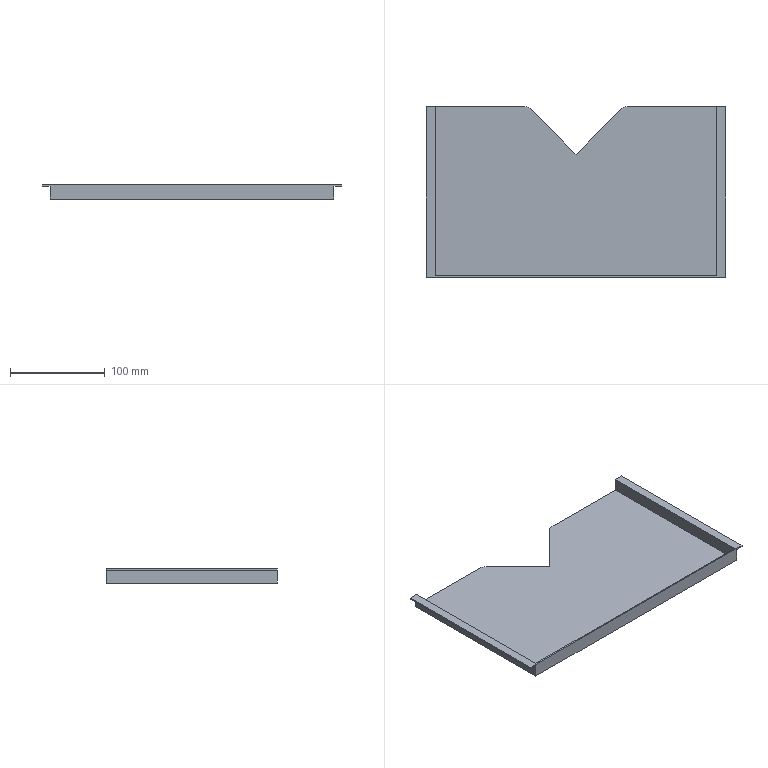Part | STEP file | 1 solid | 19 faces | box 316 x 180 x 15 mm | volume 94868 mm3 | plane 17 | cylinder 2 | commonest cylinder face diameters 20 x2
STEP:
#1=CARTESIAN_POINT('',(0.,0.,0.));
#2=DIRECTION('',(0.,0.,1.));
#3=DIRECTION('',(1.,0.,0.));
#4=AXIS2_PLACEMENT_3D('',#1,#2,#3);
#5=CARTESIAN_POINT('',(150.,90.,-15.));
#6=VERTEX_POINT('',#5);
#7=CARTESIAN_POINT('',(54.142,90.,-15.));
#8=VERTEX_POINT('',#7);
#9=CARTESIAN_POINT('',(158.,90.,-15.));
#10=DIRECTION('',(-1.,0.,0.));
#11=VECTOR('',#10,1.);
#12=LINE('',#9,#11);
#13=CARTESIAN_POINT('',(158.,-90.,-15.));
#14=DIRECTION('',(0.,0.,1.));
#15=DIRECTION('',(1.,0.,0.));
#16=AXIS2_PLACEMENT_3D('',#13,#14,#15);
#17=PLANE('',#16);
#18=CARTESIAN_POINT('',(0.,180.));
#19=DIRECTION('',(-1.,0.));
#20=VECTOR('',#19,1.);
#21=LINE('',#18,#20);
#22=(GEOMETRIC_REPRESENTATION_CONTEXT(2)PARAMETRIC_REPRESENTATION_CONTEXT()REPRESENTATION_CONTEXT('',''));
#23=DEFINITIONAL_REPRESENTATION('',(#21),#22);
#24=PCURVE('',#17,#23);
#25=CARTESIAN_POINT('',(-158.,90.,-15.));
#26=DIRECTION('',(0.,1.,0.));
#27=DIRECTION('',(0.,0.,1.));
#28=AXIS2_PLACEMENT_3D('',#25,#26,#27);
#29=PLANE('',#28);
#30=CARTESIAN_POINT('',(0.,316.));
#31=DIRECTION('',(0.,-1.));
#32=VECTOR('',#31,1.);
#33=LINE('',#30,#32);
#34=(GEOMETRIC_REPRESENTATION_CONTEXT(2)PARAMETRIC_REPRESENTATION_CONTEXT()REPRESENTATION_CONTEXT('',''));
#35=DEFINITIONAL_REPRESENTATION('',(#33),#34);
#36=PCURVE('',#29,#35);
#37=SURFACE_CURVE('',#12,(#24,#36),.PCURVE_S1.);
#38=EDGE_CURVE('',#6,#8,#37,.T.);
#39=ORIENTED_EDGE('',*,*,#38,.F.);
#40=CARTESIAN_POINT('',(150.,-90.,-15.));
#41=VERTEX_POINT('',#40);
#42=CARTESIAN_POINT('',(150.,-90.,-15.));
#43=DIRECTION('',(0.,1.,0.));
#44=VECTOR('',#43,1.);
#45=LINE('',#42,#44);
#46=CARTESIAN_POINT('',(-8.,0.));
#47=DIRECTION('',(0.,1.));
#48=VECTOR('',#47,1.);
#49=LINE('',#46,#48);
#50=(GEOMETRIC_REPRESENTATION_CONTEXT(2)PARAMETRIC_REPRESENTATION_CONTEXT()REPRESENTATION_CONTEXT('',''));
#51=DEFINITIONAL_REPRESENTATION('',(#49),#50);
#52=PCURVE('',#17,#51);
#53=CARTESIAN_POINT('',(150.,109.,-15.));
#54=DIRECTION('',(-1.,0.,0.));
#55=DIRECTION('',(0.,0.,1.));
#56=AXIS2_PLACEMENT_3D('',#53,#54,#55);
#57=PLANE('',#56);
#58=CARTESIAN_POINT('',(0.,-199.));
#59=DIRECTION('',(0.,1.));
#60=VECTOR('',#59,1.);
#61=LINE('',#58,#60);
#62=(GEOMETRIC_REPRESENTATION_CONTEXT(2)PARAMETRIC_REPRESENTATION_CONTEXT()REPRESENTATION_CONTEXT('',''));
#63=DEFINITIONAL_REPRESENTATION('',(#61),#62);
#64=PCURVE('',#57,#63);
#65=SURFACE_CURVE('',#45,(#52,#64),.PCURVE_S1.);
#66=EDGE_CURVE('',#41,#6,#65,.T.);
#67=ORIENTED_EDGE('',*,*,#66,.F.);
#68=CARTESIAN_POINT('',(-150.,-90.,-15.));
#69=VERTEX_POINT('',#68);
#70=CARTESIAN_POINT('',(158.,-90.,-15.));
#71=DIRECTION('',(1.,0.,0.));
#72=VECTOR('',#71,1.);
#73=LINE('',#70,#72);
#74=CARTESIAN_POINT('',(0.,0.));
#75=DIRECTION('',(1.,0.));
#76=VECTOR('',#75,1.);
#77=LINE('',#74,#76);
#78=(GEOMETRIC_REPRESENTATION_CONTEXT(2)PARAMETRIC_REPRESENTATION_CONTEXT()REPRESENTATION_CONTEXT('',''));
#79=DEFINITIONAL_REPRESENTATION('',(#77),#78);
#80=PCURVE('',#17,#79);
#81=CARTESIAN_POINT('',(-158.,-90.,-15.));
#82=DIRECTION('',(0.,-1.,0.));
#83=DIRECTION('',(0.,0.,-1.));
#84=AXIS2_PLACEMENT_3D('',#81,#82,#83);
#85=PLANE('',#84);
#86=CARTESIAN_POINT('',(0.,316.));
#87=DIRECTION('',(0.,1.));
#88=VECTOR('',#87,1.);
#89=LINE('',#86,#88);
#90=(GEOMETRIC_REPRESENTATION_CONTEXT(2)PARAMETRIC_REPRESENTATION_CONTEXT()REPRESENTATION_CONTEXT('',''));
#91=DEFINITIONAL_REPRESENTATION('',(#89),#90);
#92=PCURVE('',#85,#91);
#93=SURFACE_CURVE('',#73,(#80,#92),.PCURVE_S1.);
#94=EDGE_CURVE('',#69,#41,#93,.T.);
#95=ORIENTED_EDGE('',*,*,#94,.F.);
#96=CARTESIAN_POINT('',(-150.,90.,-15.));
#97=VERTEX_POINT('',#96);
#98=CARTESIAN_POINT('',(-150.,-90.,-15.));
#99=DIRECTION('',(0.,-1.,0.));
#100=VECTOR('',#99,1.);
#101=LINE('',#98,#100);
#102=CARTESIAN_POINT('',(-308.,0.));
#103=DIRECTION('',(0.,-1.));
#104=VECTOR('',#103,1.);
#105=LINE('',#102,#104);
#106=(GEOMETRIC_REPRESENTATION_CONTEXT(2)PARAMETRIC_REPRESENTATION_CONTEXT()REPRESENTATION_CONTEXT('',''));
#107=DEFINITIONAL_REPRESENTATION('',(#105),#106);
#108=PCURVE('',#17,#107);
#109=CARTESIAN_POINT('',(-150.,109.,-15.));
#110=DIRECTION('',(-1.,0.,0.));
#111=DIRECTION('',(0.,0.,1.));
#112=AXIS2_PLACEMENT_3D('',#109,#110,#111);
#113=PLANE('',#112);
#114=CARTESIAN_POINT('',(0.,-199.));
#115=DIRECTION('',(0.,-1.));
#116=VECTOR('',#115,1.);
#117=LINE('',#114,#116);
#118=(GEOMETRIC_REPRESENTATION_CONTEXT(2)PARAMETRIC_REPRESENTATION_CONTEXT()REPRESENTATION_CONTEXT('',''));
#119=DEFINITIONAL_REPRESENTATION('',(#117),#118);
#120=PCURVE('',#113,#119);
#121=SURFACE_CURVE('',#101,(#108,#120),.PCURVE_S1.);
#122=EDGE_CURVE('',#97,#69,#121,.T.);
#123=ORIENTED_EDGE('',*,*,#122,.F.);
#124=CARTESIAN_POINT('',(-54.142,90.,-15.));
#125=VERTEX_POINT('',#124);
#126=CARTESIAN_POINT('',(158.,90.,-15.));
#127=DIRECTION('',(-1.,0.,0.));
#128=VECTOR('',#127,1.);
#129=LINE('',#126,#128);
#130=CARTESIAN_POINT('',(0.,180.));
#131=DIRECTION('',(-1.,0.));
#132=VECTOR('',#131,1.);
#133=LINE('',#130,#132);
#134=(GEOMETRIC_REPRESENTATION_CONTEXT(2)PARAMETRIC_REPRESENTATION_CONTEXT()REPRESENTATION_CONTEXT('',''));
#135=DEFINITIONAL_REPRESENTATION('',(#133),#134);
#136=PCURVE('',#17,#135);
#137=CARTESIAN_POINT('',(-158.,90.,-15.));
#138=DIRECTION('',(0.,1.,0.));
#139=DIRECTION('',(0.,0.,1.));
#140=AXIS2_PLACEMENT_3D('',#137,#138,#139);
#141=PLANE('',#140);
#142=CARTESIAN_POINT('',(0.,316.));
#143=DIRECTION('',(0.,-1.));
#144=VECTOR('',#143,1.);
#145=LINE('',#142,#144);
#146=(GEOMETRIC_REPRESENTATION_CONTEXT(2)PARAMETRIC_REPRESENTATION_CONTEXT()REPRESENTATION_CONTEXT('',''));
#147=DEFINITIONAL_REPRESENTATION('',(#145),#146);
#148=PCURVE('',#141,#147);
#149=SURFACE_CURVE('',#129,(#136,#148),.PCURVE_S1.);
#150=EDGE_CURVE('',#125,#97,#149,.T.);
#151=ORIENTED_EDGE('',*,*,#150,.F.);
#152=CARTESIAN_POINT('',(-47.071,87.071,-15.));
#153=VERTEX_POINT('',#152);
#154=CARTESIAN_POINT('',(-54.142,80.,-15.));
#155=DIRECTION('',(0.,0.,1.));
#156=DIRECTION('',(1.,0.,0.));
#157=AXIS2_PLACEMENT_3D('',#154,#155,#156);
#158=CIRCLE('',#157,10.);
#159=CARTESIAN_POINT('',(-212.142,170.));
#160=DIRECTION('',(1.,0.));
#161=AXIS2_PLACEMENT_2D('',#159,#160);
#162=CIRCLE('',#161,10.);
#163=(GEOMETRIC_REPRESENTATION_CONTEXT(2)PARAMETRIC_REPRESENTATION_CONTEXT()REPRESENTATION_CONTEXT('',''));
#164=DEFINITIONAL_REPRESENTATION('',(#162),#163);
#165=PCURVE('',#17,#164);
#166=CARTESIAN_POINT('',(-54.142,80.,-488.724));
#167=DIRECTION('',(0.,0.,1.));
#168=DIRECTION('',(1.,0.,0.));
#169=AXIS2_PLACEMENT_3D('',#166,#167,#168);
#170=CYLINDRICAL_SURFACE('',#169,10.);
#171=CARTESIAN_POINT('',(0.,473.724));
#172=DIRECTION('',(1.,0.));
#173=VECTOR('',#172,1.);
#174=LINE('',#171,#173);
#175=(GEOMETRIC_REPRESENTATION_CONTEXT(2)PARAMETRIC_REPRESENTATION_CONTEXT()REPRESENTATION_CONTEXT('',''));
#176=DEFINITIONAL_REPRESENTATION('',(#174),#175);
#177=PCURVE('',#170,#176);
#178=SURFACE_CURVE('',#158,(#165,#177),.PCURVE_S1.);
#179=EDGE_CURVE('',#153,#125,#178,.T.);
#180=ORIENTED_EDGE('',*,*,#179,.F.);
#181=CARTESIAN_POINT('',(0.,40.,-15.));
#182=VERTEX_POINT('',#181);
#183=CARTESIAN_POINT('',(0.,40.,-15.));
#184=DIRECTION('',(-0.7071,0.7071,0.));
#185=VECTOR('',#184,1.);
#186=LINE('',#183,#185);
#187=CARTESIAN_POINT('',(-158.,130.));
#188=DIRECTION('',(-0.7071,0.7071));
#189=VECTOR('',#188,1.);
#190=LINE('',#187,#189);
#191=(GEOMETRIC_REPRESENTATION_CONTEXT(2)PARAMETRIC_REPRESENTATION_CONTEXT()REPRESENTATION_CONTEXT('',''));
#192=DEFINITIONAL_REPRESENTATION('',(#190),#191);
#193=PCURVE('',#17,#192);
#194=CARTESIAN_POINT('',(0.,40.,-488.724));
#195=DIRECTION('',(-0.7071,-0.7071,0.));
#196=DIRECTION('',(0.7071,-0.7071,0.));
#197=AXIS2_PLACEMENT_3D('',#194,#195,#196);
#198=PLANE('',#197);
#199=CARTESIAN_POINT('',(0.,473.724));
#200=DIRECTION('',(-1.,0.));
#201=VECTOR('',#200,1.);
#202=LINE('',#199,#201);
#203=(GEOMETRIC_REPRESENTATION_CONTEXT(2)PARAMETRIC_REPRESENTATION_CONTEXT()REPRESENTATION_CONTEXT('',''));
#204=DEFINITIONAL_REPRESENTATION('',(#202),#203);
#205=PCURVE('',#198,#204);
#206=SURFACE_CURVE('',#186,(#193,#205),.PCURVE_S1.);
#207=EDGE_CURVE('',#182,#153,#206,.T.);
#208=ORIENTED_EDGE('',*,*,#207,.F.);
#209=CARTESIAN_POINT('',(47.071,87.071,-15.));
#210=VERTEX_POINT('',#209);
#211=CARTESIAN_POINT('',(47.071,87.071,-15.));
#212=DIRECTION('',(-0.7071,-0.7071,0.));
#213=VECTOR('',#212,1.);
#214=LINE('',#211,#213);
#215=CARTESIAN_POINT('',(-110.929,177.071));
#216=DIRECTION('',(-0.7071,-0.7071));
#217=VECTOR('',#216,1.);
#218=LINE('',#215,#217);
#219=(GEOMETRIC_REPRESENTATION_CONTEXT(2)PARAMETRIC_REPRESENTATION_CONTEXT()REPRESENTATION_CONTEXT('',''));
#220=DEFINITIONAL_REPRESENTATION('',(#218),#219);
#221=PCURVE('',#17,#220);
#222=CARTESIAN_POINT('',(0.,40.,-488.724));
#223=DIRECTION('',(0.7071,-0.7071,0.));
#224=DIRECTION('',(0.7071,0.7071,0.));
#225=AXIS2_PLACEMENT_3D('',#222,#223,#224);
#226=PLANE('',#225);
#227=CARTESIAN_POINT('',(66.569,473.724));
#228=DIRECTION('',(-1.,0.));
#229=VECTOR('',#228,1.);
#230=LINE('',#227,#229);
#231=(GEOMETRIC_REPRESENTATION_CONTEXT(2)PARAMETRIC_REPRESENTATION_CONTEXT()REPRESENTATION_CONTEXT('',''));
#232=DEFINITIONAL_REPRESENTATION('',(#230),#231);
#233=PCURVE('',#226,#232);
#234=SURFACE_CURVE('',#214,(#221,#233),.PCURVE_S1.);
#235=EDGE_CURVE('',#210,#182,#234,.T.);
#236=ORIENTED_EDGE('',*,*,#235,.F.);
#237=CARTESIAN_POINT('',(54.142,80.,-15.));
#238=DIRECTION('',(0.,0.,1.));
#239=DIRECTION('',(1.,0.,0.));
#240=AXIS2_PLACEMENT_3D('',#237,#238,#239);
#241=CIRCLE('',#240,10.);
#242=CARTESIAN_POINT('',(-103.858,170.));
#243=DIRECTION('',(1.,0.));
#244=AXIS2_PLACEMENT_2D('',#242,#243);
#245=CIRCLE('',#244,10.);
#246=(GEOMETRIC_REPRESENTATION_CONTEXT(2)PARAMETRIC_REPRESENTATION_CONTEXT()REPRESENTATION_CONTEXT('',''));
#247=DEFINITIONAL_REPRESENTATION('',(#245),#246);
#248=PCURVE('',#17,#247);
#249=CARTESIAN_POINT('',(54.142,80.,-15.));
#250=DIRECTION('',(0.,0.,1.));
#251=DIRECTION('',(1.,0.,0.));
#252=AXIS2_PLACEMENT_3D('',#249,#250,#251);
#253=CYLINDRICAL_SURFACE('',#252,10.);
#254=CARTESIAN_POINT('',(0.,0.));
#255=DIRECTION('',(1.,0.));
#256=VECTOR('',#255,1.);
#257=LINE('',#254,#256);
#258=(GEOMETRIC_REPRESENTATION_CONTEXT(2)PARAMETRIC_REPRESENTATION_CONTEXT()REPRESENTATION_CONTEXT('',''));
#259=DEFINITIONAL_REPRESENTATION('',(#257),#258);
#260=PCURVE('',#253,#259);
#261=SURFACE_CURVE('',#241,(#248,#260),.PCURVE_S1.);
#262=EDGE_CURVE('',#8,#210,#261,.T.);
#263=ORIENTED_EDGE('',*,*,#262,.F.);
#264=EDGE_LOOP('',(#39,#67,#95,#123,#151,#180,#208,#236,#263));
#265=FACE_BOUND('',#264,.T.);
#266=ADVANCED_FACE('',(#265),#17,.F.);
#267=ORIENTED_EDGE('',*,*,#262,.T.);
#268=CARTESIAN_POINT('',(47.071,87.071,-13.5));
#269=VERTEX_POINT('',#268);
#270=CARTESIAN_POINT('',(47.071,87.071,-15.));
#271=DIRECTION('',(0.,0.,1.));
#272=VECTOR('',#271,1.);
#273=LINE('',#270,#272);
#274=CARTESIAN_POINT('',(2.356,0.));
#275=DIRECTION('',(0.,1.));
#276=VECTOR('',#275,1.);
#277=LINE('',#274,#276);
#278=(GEOMETRIC_REPRESENTATION_CONTEXT(2)PARAMETRIC_REPRESENTATION_CONTEXT()REPRESENTATION_CONTEXT('',''));
#279=DEFINITIONAL_REPRESENTATION('',(#277),#278);
#280=PCURVE('',#253,#279);
#281=CARTESIAN_POINT('',(66.569,473.724));
#282=DIRECTION('',(0.,1.));
#283=VECTOR('',#282,1.);
#284=LINE('',#281,#283);
#285=(GEOMETRIC_REPRESENTATION_CONTEXT(2)PARAMETRIC_REPRESENTATION_CONTEXT()REPRESENTATION_CONTEXT('',''));
#286=DEFINITIONAL_REPRESENTATION('',(#284),#285);
#287=PCURVE('',#226,#286);
#288=SURFACE_CURVE('',#273,(#280,#287),.PCURVE_S1.);
#289=EDGE_CURVE('',#210,#269,#288,.T.);
#290=ORIENTED_EDGE('',*,*,#289,.T.);
#291=CARTESIAN_POINT('',(54.142,90.,-13.5));
#292=VERTEX_POINT('',#291);
#293=CARTESIAN_POINT('',(54.142,80.,-13.5));
#294=DIRECTION('',(0.,0.,-1.));
#295=DIRECTION('',(1.,0.,0.));
#296=AXIS2_PLACEMENT_3D('',#293,#294,#295);
#297=CIRCLE('',#296,10.);
#298=CARTESIAN_POINT('',(6.283,1.5));
#299=DIRECTION('',(-1.,0.));
#300=VECTOR('',#299,1.);
#301=LINE('',#298,#300);
#302=(GEOMETRIC_REPRESENTATION_CONTEXT(2)PARAMETRIC_REPRESENTATION_CONTEXT()REPRESENTATION_CONTEXT('',''));
#303=DEFINITIONAL_REPRESENTATION('',(#301),#302);
#304=PCURVE('',#253,#303);
#305=CARTESIAN_POINT('',(158.,-90.,-13.5));
#306=DIRECTION('',(0.,0.,1.));
#307=DIRECTION('',(1.,0.,0.));
#308=AXIS2_PLACEMENT_3D('',#305,#306,#307);
#309=PLANE('',#308);
#310=CARTESIAN_POINT('',(-93.858,170.));
#311=CARTESIAN_POINT('',(-93.858,152.679));
#312=CARTESIAN_POINT('',(-108.858,161.34));
#313=CARTESIAN_POINT('',(-123.858,170.));
#314=CARTESIAN_POINT('',(-108.858,178.66));
#315=CARTESIAN_POINT('',(-93.858,187.321));
#316=CARTESIAN_POINT('',(-93.858,170.));
#317=(BOUNDED_CURVE()B_SPLINE_CURVE(2,(#310,#311,#312,#313,#314,#315,#316),.UNSPECIFIED.,.T.,.F.)B_SPLINE_CURVE_WITH_KNOTS((1,2,2,2,2,1),(-2.094,0.,2.094,4.189,6.283,8.378),.UNSPECIFIED.)CURVE()GEOMETRIC_REPRESENTATION_ITEM()RATIONAL_B_SPLINE_CURVE((1.,0.5,1.,0.5,1.,0.5,1.))REPRESENTATION_ITEM(''));
#318=(GEOMETRIC_REPRESENTATION_CONTEXT(2)PARAMETRIC_REPRESENTATION_CONTEXT()REPRESENTATION_CONTEXT('',''));
#319=DEFINITIONAL_REPRESENTATION('',(#317),#318);
#320=PCURVE('',#309,#319);
#321=SURFACE_CURVE('',#297,(#304,#320),.PCURVE_S1.);
#322=EDGE_CURVE('',#269,#292,#321,.T.);
#323=ORIENTED_EDGE('',*,*,#322,.T.);
#324=CARTESIAN_POINT('',(54.142,90.,-15.));
#325=DIRECTION('',(0.,0.,-1.));
#326=VECTOR('',#325,1.);
#327=LINE('',#324,#326);
#328=CARTESIAN_POINT('',(1.571,0.));
#329=DIRECTION('',(0.,-1.));
#330=VECTOR('',#329,1.);
#331=LINE('',#328,#330);
#332=(GEOMETRIC_REPRESENTATION_CONTEXT(2)PARAMETRIC_REPRESENTATION_CONTEXT()REPRESENTATION_CONTEXT('',''));
#333=DEFINITIONAL_REPRESENTATION('',(#331),#332);
#334=PCURVE('',#253,#333);
#335=CARTESIAN_POINT('',(0.,212.142));
#336=DIRECTION('',(-1.,0.));
#337=VECTOR('',#336,1.);
#338=LINE('',#335,#337);
#339=(GEOMETRIC_REPRESENTATION_CONTEXT(2)PARAMETRIC_REPRESENTATION_CONTEXT()REPRESENTATION_CONTEXT('',''));
#340=DEFINITIONAL_REPRESENTATION('',(#338),#339);
#341=PCURVE('',#29,#340);
#342=SURFACE_CURVE('',#327,(#334,#341),.PCURVE_S1.);
#343=EDGE_CURVE('',#292,#8,#342,.T.);
#344=ORIENTED_EDGE('',*,*,#343,.T.);
#345=EDGE_LOOP('',(#267,#290,#323,#344));
#346=FACE_BOUND('',#345,.T.);
#347=ADVANCED_FACE('',(#346),#253,.T.);
#348=CARTESIAN_POINT('',(148.5,90.,0.));
#349=VERTEX_POINT('',#348);
#350=CARTESIAN_POINT('',(158.,90.,0.));
#351=VERTEX_POINT('',#350);
#352=CARTESIAN_POINT('',(-158.,90.,0.));
#353=DIRECTION('',(1.,0.,0.));
#354=VECTOR('',#353,1.);
#355=LINE('',#352,#354);
#356=CARTESIAN_POINT('',(15.,0.));
#357=DIRECTION('',(0.,1.));
#358=VECTOR('',#357,1.);
#359=LINE('',#356,#358);
#360=(GEOMETRIC_REPRESENTATION_CONTEXT(2)PARAMETRIC_REPRESENTATION_CONTEXT()REPRESENTATION_CONTEXT('',''));
#361=DEFINITIONAL_REPRESENTATION('',(#359),#360);
#362=PCURVE('',#29,#361);
#363=CARTESIAN_POINT('',(158.,-90.,0.));
#364=DIRECTION('',(0.,0.,1.));
#365=DIRECTION('',(1.,0.,0.));
#366=AXIS2_PLACEMENT_3D('',#363,#364,#365);
#367=PLANE('',#366);
#368=CARTESIAN_POINT('',(-316.,180.));
#369=DIRECTION('',(1.,0.));
#370=VECTOR('',#369,1.);
#371=LINE('',#368,#370);
#372=(GEOMETRIC_REPRESENTATION_CONTEXT(2)PARAMETRIC_REPRESENTATION_CONTEXT()REPRESENTATION_CONTEXT('',''));
#373=DEFINITIONAL_REPRESENTATION('',(#371),#372);
#374=PCURVE('',#367,#373);
#375=SURFACE_CURVE('',#355,(#362,#374),.PCURVE_S1.);
#376=EDGE_CURVE('',#349,#351,#375,.T.);
#377=ORIENTED_EDGE('',*,*,#376,.T.);
#378=CARTESIAN_POINT('',(158.,90.,-1.5));
#379=VERTEX_POINT('',#378);
#380=CARTESIAN_POINT('',(158.,90.,-15.));
#381=DIRECTION('',(0.,0.,1.));
#382=VECTOR('',#381,1.);
#383=LINE('',#380,#382);
#384=CARTESIAN_POINT('',(0.,316.));
#385=DIRECTION('',(1.,0.));
#386=VECTOR('',#385,1.);
#387=LINE('',#384,#386);
#388=(GEOMETRIC_REPRESENTATION_CONTEXT(2)PARAMETRIC_REPRESENTATION_CONTEXT()REPRESENTATION_CONTEXT('',''));
#389=DEFINITIONAL_REPRESENTATION('',(#387),#388);
#390=PCURVE('',#29,#389);
#391=CARTESIAN_POINT('',(158.,90.,-15.));
#392=DIRECTION('',(1.,0.,0.));
#393=DIRECTION('',(0.,0.,-1.));
#394=AXIS2_PLACEMENT_3D('',#391,#392,#393);
#395=PLANE('',#394);
#396=CARTESIAN_POINT('',(0.,0.));
#397=DIRECTION('',(-1.,0.));
#398=VECTOR('',#397,1.);
#399=LINE('',#396,#398);
#400=(GEOMETRIC_REPRESENTATION_CONTEXT(2)PARAMETRIC_REPRESENTATION_CONTEXT()REPRESENTATION_CONTEXT('',''));
#401=DEFINITIONAL_REPRESENTATION('',(#399),#400);
#402=PCURVE('',#395,#401);
#403=SURFACE_CURVE('',#383,(#390,#402),.PCURVE_S1.);
#404=EDGE_CURVE('',#379,#351,#403,.T.);
#405=ORIENTED_EDGE('',*,*,#404,.F.);
#406=CARTESIAN_POINT('',(150.,90.,-1.5));
#407=VERTEX_POINT('',#406);
#408=CARTESIAN_POINT('',(-158.,90.,-1.5));
#409=DIRECTION('',(-1.,0.,0.));
#410=VECTOR('',#409,1.);
#411=LINE('',#408,#410);
#412=CARTESIAN_POINT('',(13.5,0.));
#413=DIRECTION('',(0.,-1.));
#414=VECTOR('',#413,1.);
#415=LINE('',#412,#414);
#416=(GEOMETRIC_REPRESENTATION_CONTEXT(2)PARAMETRIC_REPRESENTATION_CONTEXT()REPRESENTATION_CONTEXT('',''));
#417=DEFINITIONAL_REPRESENTATION('',(#415),#416);
#418=PCURVE('',#29,#417);
#419=CARTESIAN_POINT('',(158.,109.,-1.5));
#420=DIRECTION('',(0.,0.,1.));
#421=DIRECTION('',(1.,0.,0.));
#422=AXIS2_PLACEMENT_3D('',#419,#420,#421);
#423=PLANE('',#422);
#424=CARTESIAN_POINT('',(-316.,-19.));
#425=DIRECTION('',(-1.,0.));
#426=VECTOR('',#425,1.);
#427=LINE('',#424,#426);
#428=(GEOMETRIC_REPRESENTATION_CONTEXT(2)PARAMETRIC_REPRESENTATION_CONTEXT()REPRESENTATION_CONTEXT('',''));
#429=DEFINITIONAL_REPRESENTATION('',(#427),#428);
#430=PCURVE('',#423,#429);
#431=SURFACE_CURVE('',#411,(#418,#430),.PCURVE_S1.);
#432=EDGE_CURVE('',#379,#407,#431,.T.);
#433=ORIENTED_EDGE('',*,*,#432,.T.);
#434=CARTESIAN_POINT('',(150.,90.,-15.));
#435=DIRECTION('',(0.,0.,-1.));
#436=VECTOR('',#435,1.);
#437=LINE('',#434,#436);
#438=CARTESIAN_POINT('',(0.,308.));
#439=DIRECTION('',(-1.,0.));
#440=VECTOR('',#439,1.);
#441=LINE('',#438,#440);
#442=(GEOMETRIC_REPRESENTATION_CONTEXT(2)PARAMETRIC_REPRESENTATION_CONTEXT()REPRESENTATION_CONTEXT('',''));
#443=DEFINITIONAL_REPRESENTATION('',(#441),#442);
#444=PCURVE('',#29,#443);
#445=CARTESIAN_POINT('',(0.,-19.));
#446=DIRECTION('',(-1.,0.));
#447=VECTOR('',#446,1.);
#448=LINE('',#445,#447);
#449=(GEOMETRIC_REPRESENTATION_CONTEXT(2)PARAMETRIC_REPRESENTATION_CONTEXT()REPRESENTATION_CONTEXT('',''));
#450=DEFINITIONAL_REPRESENTATION('',(#448),#449);
#451=PCURVE('',#57,#450);
#452=SURFACE_CURVE('',#437,(#444,#451),.PCURVE_S1.);
#453=EDGE_CURVE('',#407,#6,#452,.T.);
#454=ORIENTED_EDGE('',*,*,#453,.T.);
#455=ORIENTED_EDGE('',*,*,#38,.T.);
#456=ORIENTED_EDGE('',*,*,#343,.F.);
#457=CARTESIAN_POINT('',(148.5,90.,-13.5));
#458=VERTEX_POINT('',#457);
#459=CARTESIAN_POINT('',(-158.,90.,-13.5));
#460=DIRECTION('',(1.,0.,0.));
#461=VECTOR('',#460,1.);
#462=LINE('',#459,#461);
#463=CARTESIAN_POINT('',(1.5,0.));
#464=DIRECTION('',(0.,1.));
#465=VECTOR('',#464,1.);
#466=LINE('',#463,#465);
#467=(GEOMETRIC_REPRESENTATION_CONTEXT(2)PARAMETRIC_REPRESENTATION_CONTEXT()REPRESENTATION_CONTEXT('',''));
#468=DEFINITIONAL_REPRESENTATION('',(#466),#467);
#469=PCURVE('',#29,#468);
#470=CARTESIAN_POINT('',(-316.,180.));
#471=DIRECTION('',(1.,0.));
#472=VECTOR('',#471,1.);
#473=LINE('',#470,#472);
#474=(GEOMETRIC_REPRESENTATION_CONTEXT(2)PARAMETRIC_REPRESENTATION_CONTEXT()REPRESENTATION_CONTEXT('',''));
#475=DEFINITIONAL_REPRESENTATION('',(#473),#474);
#476=PCURVE('',#309,#475);
#477=SURFACE_CURVE('',#462,(#469,#476),.PCURVE_S1.);
#478=EDGE_CURVE('',#292,#458,#477,.T.);
#479=ORIENTED_EDGE('',*,*,#478,.T.);
#480=CARTESIAN_POINT('',(148.5,90.,-15.));
#481=DIRECTION('',(0.,0.,1.));
#482=VECTOR('',#481,1.);
#483=LINE('',#480,#482);
#484=CARTESIAN_POINT('',(0.,306.5));
#485=DIRECTION('',(1.,0.));
#486=VECTOR('',#485,1.);
#487=LINE('',#484,#486);
#488=(GEOMETRIC_REPRESENTATION_CONTEXT(2)PARAMETRIC_REPRESENTATION_CONTEXT()REPRESENTATION_CONTEXT('',''));
#489=DEFINITIONAL_REPRESENTATION('',(#487),#488);
#490=PCURVE('',#29,#489);
#491=CARTESIAN_POINT('',(148.5,109.,-15.));
#492=DIRECTION('',(-1.,0.,0.));
#493=DIRECTION('',(0.,0.,1.));
#494=AXIS2_PLACEMENT_3D('',#491,#492,#493);
#495=PLANE('',#494);
#496=CARTESIAN_POINT('',(0.,-19.));
#497=DIRECTION('',(1.,0.));
#498=VECTOR('',#497,1.);
#499=LINE('',#496,#498);
#500=(GEOMETRIC_REPRESENTATION_CONTEXT(2)PARAMETRIC_REPRESENTATION_CONTEXT()REPRESENTATION_CONTEXT('',''));
#501=DEFINITIONAL_REPRESENTATION('',(#499),#500);
#502=PCURVE('',#495,#501);
#503=SURFACE_CURVE('',#483,(#490,#502),.PCURVE_S1.);
#504=EDGE_CURVE('',#458,#349,#503,.T.);
#505=ORIENTED_EDGE('',*,*,#504,.T.);
#506=EDGE_LOOP('',(#377,#405,#433,#454,#455,#456,#479,#505));
#507=FACE_BOUND('',#506,.T.);
#508=ADVANCED_FACE('',(#507),#29,.T.);
#509=CARTESIAN_POINT('',(150.,-90.,-1.5));
#510=VERTEX_POINT('',#509);
#511=CARTESIAN_POINT('',(150.,-90.,-15.));
#512=DIRECTION('',(0.,0.,1.));
#513=VECTOR('',#512,1.);
#514=LINE('',#511,#513);
#515=CARTESIAN_POINT('',(0.,-199.));
#516=DIRECTION('',(1.,0.));
#517=VECTOR('',#516,1.);
#518=LINE('',#515,#517);
#519=(GEOMETRIC_REPRESENTATION_CONTEXT(2)PARAMETRIC_REPRESENTATION_CONTEXT()REPRESENTATION_CONTEXT('',''));
#520=DEFINITIONAL_REPRESENTATION('',(#518),#519);
#521=PCURVE('',#57,#520);
#522=CARTESIAN_POINT('',(0.,308.));
#523=DIRECTION('',(-1.,0.));
#524=VECTOR('',#523,1.);
#525=LINE('',#522,#524);
#526=(GEOMETRIC_REPRESENTATION_CONTEXT(2)PARAMETRIC_REPRESENTATION_CONTEXT()REPRESENTATION_CONTEXT('',''));
#527=DEFINITIONAL_REPRESENTATION('',(#525),#526);
#528=PCURVE('',#85,#527);
#529=SURFACE_CURVE('',#514,(#521,#528),.PCURVE_S1.);
#530=EDGE_CURVE('',#41,#510,#529,.T.);
#531=ORIENTED_EDGE('',*,*,#530,.F.);
#532=ORIENTED_EDGE('',*,*,#66,.T.);
#533=ORIENTED_EDGE('',*,*,#453,.F.);
#534=CARTESIAN_POINT('',(150.,109.,-1.5));
#535=DIRECTION('',(0.,1.,0.));
#536=VECTOR('',#535,1.);
#537=LINE('',#534,#536);
#538=CARTESIAN_POINT('',(13.5,0.));
#539=DIRECTION('',(0.,1.));
#540=VECTOR('',#539,1.);
#541=LINE('',#538,#540);
#542=(GEOMETRIC_REPRESENTATION_CONTEXT(2)PARAMETRIC_REPRESENTATION_CONTEXT()REPRESENTATION_CONTEXT('',''));
#543=DEFINITIONAL_REPRESENTATION('',(#541),#542);
#544=PCURVE('',#57,#543);
#545=CARTESIAN_POINT('',(-8.,0.));
#546=DIRECTION('',(0.,1.));
#547=VECTOR('',#546,1.);
#548=LINE('',#545,#547);
#549=(GEOMETRIC_REPRESENTATION_CONTEXT(2)PARAMETRIC_REPRESENTATION_CONTEXT()REPRESENTATION_CONTEXT('',''));
#550=DEFINITIONAL_REPRESENTATION('',(#548),#549);
#551=PCURVE('',#423,#550);
#552=SURFACE_CURVE('',#537,(#544,#551),.PCURVE_S1.);
#553=EDGE_CURVE('',#510,#407,#552,.T.);
#554=ORIENTED_EDGE('',*,*,#553,.F.);
#555=EDGE_LOOP('',(#531,#532,#533,#554));
#556=FACE_BOUND('',#555,.T.);
#557=ADVANCED_FACE('',(#556),#57,.F.);
#558=ORIENTED_EDGE('',*,*,#530,.T.);
#559=CARTESIAN_POINT('',(158.,-90.,-1.5));
#560=VERTEX_POINT('',#559);
#561=CARTESIAN_POINT('',(-158.,-90.,-1.5));
#562=DIRECTION('',(1.,0.,0.));
#563=VECTOR('',#562,1.);
#564=LINE('',#561,#563);
#565=CARTESIAN_POINT('',(-13.5,0.));
#566=DIRECTION('',(0.,1.));
#567=VECTOR('',#566,1.);
#568=LINE('',#565,#567);
#569=(GEOMETRIC_REPRESENTATION_CONTEXT(2)PARAMETRIC_REPRESENTATION_CONTEXT()REPRESENTATION_CONTEXT('',''));
#570=DEFINITIONAL_REPRESENTATION('',(#568),#569);
#571=PCURVE('',#85,#570);
#572=CARTESIAN_POINT('',(-316.,-199.));
#573=DIRECTION('',(1.,0.));
#574=VECTOR('',#573,1.);
#575=LINE('',#572,#574);
#576=(GEOMETRIC_REPRESENTATION_CONTEXT(2)PARAMETRIC_REPRESENTATION_CONTEXT()REPRESENTATION_CONTEXT('',''));
#577=DEFINITIONAL_REPRESENTATION('',(#575),#576);
#578=PCURVE('',#423,#577);
#579=SURFACE_CURVE('',#564,(#571,#578),.PCURVE_S1.);
#580=EDGE_CURVE('',#510,#560,#579,.T.);
#581=ORIENTED_EDGE('',*,*,#580,.T.);
#582=CARTESIAN_POINT('',(158.,-90.,0.));
#583=VERTEX_POINT('',#582);
#584=CARTESIAN_POINT('',(158.,-90.,-15.));
#585=DIRECTION('',(0.,0.,-1.));
#586=VECTOR('',#585,1.);
#587=LINE('',#584,#586);
#588=CARTESIAN_POINT('',(0.,316.));
#589=DIRECTION('',(1.,0.));
#590=VECTOR('',#589,1.);
#591=LINE('',#588,#590);
#592=(GEOMETRIC_REPRESENTATION_CONTEXT(2)PARAMETRIC_REPRESENTATION_CONTEXT()REPRESENTATION_CONTEXT('',''));
#593=DEFINITIONAL_REPRESENTATION('',(#591),#592);
#594=PCURVE('',#85,#593);
#595=CARTESIAN_POINT('',(0.,-180.));
#596=DIRECTION('',(1.,0.));
#597=VECTOR('',#596,1.);
#598=LINE('',#595,#597);
#599=(GEOMETRIC_REPRESENTATION_CONTEXT(2)PARAMETRIC_REPRESENTATION_CONTEXT()REPRESENTATION_CONTEXT('',''));
#600=DEFINITIONAL_REPRESENTATION('',(#598),#599);
#601=PCURVE('',#395,#600);
#602=SURFACE_CURVE('',#587,(#594,#601),.PCURVE_S1.);
#603=EDGE_CURVE('',#583,#560,#602,.T.);
#604=ORIENTED_EDGE('',*,*,#603,.F.);
#605=CARTESIAN_POINT('',(-158.,-90.,0.));
#606=VERTEX_POINT('',#605);
#607=CARTESIAN_POINT('',(-158.,-90.,0.));
#608=DIRECTION('',(-1.,0.,0.));
#609=VECTOR('',#608,1.);
#610=LINE('',#607,#609);
#611=CARTESIAN_POINT('',(-15.,0.));
#612=DIRECTION('',(0.,-1.));
#613=VECTOR('',#612,1.);
#614=LINE('',#611,#613);
#615=(GEOMETRIC_REPRESENTATION_CONTEXT(2)PARAMETRIC_REPRESENTATION_CONTEXT()REPRESENTATION_CONTEXT('',''));
#616=DEFINITIONAL_REPRESENTATION('',(#614),#615);
#617=PCURVE('',#85,#616);
#618=CARTESIAN_POINT('',(-316.,0.));
#619=DIRECTION('',(-1.,0.));
#620=VECTOR('',#619,1.);
#621=LINE('',#618,#620);
#622=(GEOMETRIC_REPRESENTATION_CONTEXT(2)PARAMETRIC_REPRESENTATION_CONTEXT()REPRESENTATION_CONTEXT('',''));
#623=DEFINITIONAL_REPRESENTATION('',(#621),#622);
#624=PCURVE('',#367,#623);
#625=SURFACE_CURVE('',#610,(#617,#624),.PCURVE_S1.);
#626=EDGE_CURVE('',#583,#606,#625,.T.);
#627=ORIENTED_EDGE('',*,*,#626,.T.);
#628=CARTESIAN_POINT('',(-158.,-90.,-1.5));
#629=VERTEX_POINT('',#628);
#630=CARTESIAN_POINT('',(-158.,-90.,-15.));
#631=DIRECTION('',(0.,0.,1.));
#632=VECTOR('',#631,1.);
#633=LINE('',#630,#632);
#634=CARTESIAN_POINT('',(0.,0.));
#635=DIRECTION('',(-1.,0.));
#636=VECTOR('',#635,1.);
#637=LINE('',#634,#636);
#638=(GEOMETRIC_REPRESENTATION_CONTEXT(2)PARAMETRIC_REPRESENTATION_CONTEXT()REPRESENTATION_CONTEXT('',''));
#639=DEFINITIONAL_REPRESENTATION('',(#637),#638);
#640=PCURVE('',#85,#639);
#641=CARTESIAN_POINT('',(-158.,90.,-15.));
#642=DIRECTION('',(-1.,0.,0.));
#643=DIRECTION('',(0.,0.,1.));
#644=AXIS2_PLACEMENT_3D('',#641,#642,#643);
#645=PLANE('',#644);
#646=CARTESIAN_POINT('',(0.,-180.));
#647=DIRECTION('',(1.,0.));
#648=VECTOR('',#647,1.);
#649=LINE('',#646,#648);
#650=(GEOMETRIC_REPRESENTATION_CONTEXT(2)PARAMETRIC_REPRESENTATION_CONTEXT()REPRESENTATION_CONTEXT('',''));
#651=DEFINITIONAL_REPRESENTATION('',(#649),#650);
#652=PCURVE('',#645,#651);
#653=SURFACE_CURVE('',#633,(#640,#652),.PCURVE_S1.);
#654=EDGE_CURVE('',#629,#606,#653,.T.);
#655=ORIENTED_EDGE('',*,*,#654,.F.);
#656=CARTESIAN_POINT('',(-150.,-90.,-1.5));
#657=VERTEX_POINT('',#656);
#658=CARTESIAN_POINT('',(-158.,-90.,-1.5));
#659=DIRECTION('',(1.,0.,0.));
#660=VECTOR('',#659,1.);
#661=LINE('',#658,#660);
#662=CARTESIAN_POINT('',(-13.5,0.));
#663=DIRECTION('',(0.,1.));
#664=VECTOR('',#663,1.);
#665=LINE('',#662,#664);
#666=(GEOMETRIC_REPRESENTATION_CONTEXT(2)PARAMETRIC_REPRESENTATION_CONTEXT()REPRESENTATION_CONTEXT('',''));
#667=DEFINITIONAL_REPRESENTATION('',(#665),#666);
#668=PCURVE('',#85,#667);
#669=CARTESIAN_POINT('',(-158.,109.,-1.5));
#670=DIRECTION('',(0.,0.,-1.));
#671=DIRECTION('',(-1.,0.,0.));
#672=AXIS2_PLACEMENT_3D('',#669,#670,#671);
#673=PLANE('',#672);
#674=CARTESIAN_POINT('',(0.,-199.));
#675=DIRECTION('',(-1.,0.));
#676=VECTOR('',#675,1.);
#677=LINE('',#674,#676);
#678=(GEOMETRIC_REPRESENTATION_CONTEXT(2)PARAMETRIC_REPRESENTATION_CONTEXT()REPRESENTATION_CONTEXT('',''));
#679=DEFINITIONAL_REPRESENTATION('',(#677),#678);
#680=PCURVE('',#673,#679);
#681=SURFACE_CURVE('',#661,(#668,#680),.PCURVE_S1.);
#682=EDGE_CURVE('',#629,#657,#681,.T.);
#683=ORIENTED_EDGE('',*,*,#682,.T.);
#684=CARTESIAN_POINT('',(-150.,-90.,-15.));
#685=DIRECTION('',(0.,0.,-1.));
#686=VECTOR('',#685,1.);
#687=LINE('',#684,#686);
#688=CARTESIAN_POINT('',(0.,8.));
#689=DIRECTION('',(1.,0.));
#690=VECTOR('',#689,1.);
#691=LINE('',#688,#690);
#692=(GEOMETRIC_REPRESENTATION_CONTEXT(2)PARAMETRIC_REPRESENTATION_CONTEXT()REPRESENTATION_CONTEXT('',''));
#693=DEFINITIONAL_REPRESENTATION('',(#691),#692);
#694=PCURVE('',#85,#693);
#695=CARTESIAN_POINT('',(0.,-199.));
#696=DIRECTION('',(-1.,0.));
#697=VECTOR('',#696,1.);
#698=LINE('',#695,#697);
#699=(GEOMETRIC_REPRESENTATION_CONTEXT(2)PARAMETRIC_REPRESENTATION_CONTEXT()REPRESENTATION_CONTEXT('',''));
#700=DEFINITIONAL_REPRESENTATION('',(#698),#699);
#701=PCURVE('',#113,#700);
#702=SURFACE_CURVE('',#687,(#694,#701),.PCURVE_S1.);
#703=EDGE_CURVE('',#657,#69,#702,.T.);
#704=ORIENTED_EDGE('',*,*,#703,.T.);
#705=ORIENTED_EDGE('',*,*,#94,.T.);
#706=EDGE_LOOP('',(#558,#581,#604,#627,#655,#683,#704,#705));
#707=FACE_BOUND('',#706,.T.);
#708=ADVANCED_FACE('',(#707),#85,.T.);
#709=ORIENTED_EDGE('',*,*,#122,.T.);
#710=ORIENTED_EDGE('',*,*,#703,.F.);
#711=CARTESIAN_POINT('',(-150.,90.,-1.5));
#712=VERTEX_POINT('',#711);
#713=CARTESIAN_POINT('',(-150.,109.,-1.5));
#714=DIRECTION('',(0.,1.,0.));
#715=VECTOR('',#714,1.);
#716=LINE('',#713,#715);
#717=CARTESIAN_POINT('',(13.5,0.));
#718=DIRECTION('',(0.,1.));
#719=VECTOR('',#718,1.);
#720=LINE('',#717,#719);
#721=(GEOMETRIC_REPRESENTATION_CONTEXT(2)PARAMETRIC_REPRESENTATION_CONTEXT()REPRESENTATION_CONTEXT('',''));
#722=DEFINITIONAL_REPRESENTATION('',(#720),#721);
#723=PCURVE('',#113,#722);
#724=CARTESIAN_POINT('',(-8.,0.));
#725=DIRECTION('',(0.,1.));
#726=VECTOR('',#725,1.);
#727=LINE('',#724,#726);
#728=(GEOMETRIC_REPRESENTATION_CONTEXT(2)PARAMETRIC_REPRESENTATION_CONTEXT()REPRESENTATION_CONTEXT('',''));
#729=DEFINITIONAL_REPRESENTATION('',(#727),#728);
#730=PCURVE('',#673,#729);
#731=SURFACE_CURVE('',#716,(#723,#730),.PCURVE_S1.);
#732=EDGE_CURVE('',#657,#712,#731,.T.);
#733=ORIENTED_EDGE('',*,*,#732,.T.);
#734=CARTESIAN_POINT('',(-150.,90.,-15.));
#735=DIRECTION('',(0.,0.,-1.));
#736=VECTOR('',#735,1.);
#737=LINE('',#734,#736);
#738=CARTESIAN_POINT('',(0.,-19.));
#739=DIRECTION('',(-1.,0.));
#740=VECTOR('',#739,1.);
#741=LINE('',#738,#740);
#742=(GEOMETRIC_REPRESENTATION_CONTEXT(2)PARAMETRIC_REPRESENTATION_CONTEXT()REPRESENTATION_CONTEXT('',''));
#743=DEFINITIONAL_REPRESENTATION('',(#741),#742);
#744=PCURVE('',#113,#743);
#745=CARTESIAN_POINT('',(0.,8.));
#746=DIRECTION('',(-1.,0.));
#747=VECTOR('',#746,1.);
#748=LINE('',#745,#747);
#749=(GEOMETRIC_REPRESENTATION_CONTEXT(2)PARAMETRIC_REPRESENTATION_CONTEXT()REPRESENTATION_CONTEXT('',''));
#750=DEFINITIONAL_REPRESENTATION('',(#748),#749);
#751=PCURVE('',#141,#750);
#752=SURFACE_CURVE('',#737,(#744,#751),.PCURVE_S1.);
#753=EDGE_CURVE('',#712,#97,#752,.T.);
#754=ORIENTED_EDGE('',*,*,#753,.T.);
#755=EDGE_LOOP('',(#709,#710,#733,#754));
#756=FACE_BOUND('',#755,.T.);
#757=ADVANCED_FACE('',(#756),#113,.T.);
#758=CARTESIAN_POINT('',(-158.,90.,-1.5));
#759=VERTEX_POINT('',#758);
#760=CARTESIAN_POINT('',(-158.,90.,-1.5));
#761=DIRECTION('',(-1.,0.,0.));
#762=VECTOR('',#761,1.);
#763=LINE('',#760,#762);
#764=CARTESIAN_POINT('',(13.5,0.));
#765=DIRECTION('',(0.,-1.));
#766=VECTOR('',#765,1.);
#767=LINE('',#764,#766);
#768=(GEOMETRIC_REPRESENTATION_CONTEXT(2)PARAMETRIC_REPRESENTATION_CONTEXT()REPRESENTATION_CONTEXT('',''));
#769=DEFINITIONAL_REPRESENTATION('',(#767),#768);
#770=PCURVE('',#141,#769);
#771=CARTESIAN_POINT('',(0.,-19.));
#772=DIRECTION('',(1.,0.));
#773=VECTOR('',#772,1.);
#774=LINE('',#771,#773);
#775=(GEOMETRIC_REPRESENTATION_CONTEXT(2)PARAMETRIC_REPRESENTATION_CONTEXT()REPRESENTATION_CONTEXT('',''));
#776=DEFINITIONAL_REPRESENTATION('',(#774),#775);
#777=PCURVE('',#673,#776);
#778=SURFACE_CURVE('',#763,(#770,#777),.PCURVE_S1.);
#779=EDGE_CURVE('',#712,#759,#778,.T.);
#780=ORIENTED_EDGE('',*,*,#779,.T.);
#781=CARTESIAN_POINT('',(-158.,90.,0.));
#782=VERTEX_POINT('',#781);
#783=CARTESIAN_POINT('',(-158.,90.,-15.));
#784=DIRECTION('',(0.,0.,-1.));
#785=VECTOR('',#784,1.);
#786=LINE('',#783,#785);
#787=CARTESIAN_POINT('',(0.,0.));
#788=DIRECTION('',(-1.,0.));
#789=VECTOR('',#788,1.);
#790=LINE('',#787,#789);
#791=(GEOMETRIC_REPRESENTATION_CONTEXT(2)PARAMETRIC_REPRESENTATION_CONTEXT()REPRESENTATION_CONTEXT('',''));
#792=DEFINITIONAL_REPRESENTATION('',(#790),#791);
#793=PCURVE('',#141,#792);
#794=CARTESIAN_POINT('',(0.,0.));
#795=DIRECTION('',(-1.,0.));
#796=VECTOR('',#795,1.);
#797=LINE('',#794,#796);
#798=(GEOMETRIC_REPRESENTATION_CONTEXT(2)PARAMETRIC_REPRESENTATION_CONTEXT()REPRESENTATION_CONTEXT('',''));
#799=DEFINITIONAL_REPRESENTATION('',(#797),#798);
#800=PCURVE('',#645,#799);
#801=SURFACE_CURVE('',#786,(#793,#800),.PCURVE_S1.);
#802=EDGE_CURVE('',#782,#759,#801,.T.);
#803=ORIENTED_EDGE('',*,*,#802,.F.);
#804=CARTESIAN_POINT('',(-148.5,90.,0.));
#805=VERTEX_POINT('',#804);
#806=CARTESIAN_POINT('',(-158.,90.,0.));
#807=DIRECTION('',(1.,0.,0.));
#808=VECTOR('',#807,1.);
#809=LINE('',#806,#808);
#810=CARTESIAN_POINT('',(15.,0.));
#811=DIRECTION('',(0.,1.));
#812=VECTOR('',#811,1.);
#813=LINE('',#810,#812);
#814=(GEOMETRIC_REPRESENTATION_CONTEXT(2)PARAMETRIC_REPRESENTATION_CONTEXT()REPRESENTATION_CONTEXT('',''));
#815=DEFINITIONAL_REPRESENTATION('',(#813),#814);
#816=PCURVE('',#141,#815);
#817=CARTESIAN_POINT('',(-316.,180.));
#818=DIRECTION('',(1.,0.));
#819=VECTOR('',#818,1.);
#820=LINE('',#817,#819);
#821=(GEOMETRIC_REPRESENTATION_CONTEXT(2)PARAMETRIC_REPRESENTATION_CONTEXT()REPRESENTATION_CONTEXT('',''));
#822=DEFINITIONAL_REPRESENTATION('',(#820),#821);
#823=PCURVE('',#367,#822);
#824=SURFACE_CURVE('',#809,(#816,#823),.PCURVE_S1.);
#825=EDGE_CURVE('',#782,#805,#824,.T.);
#826=ORIENTED_EDGE('',*,*,#825,.T.);
#827=CARTESIAN_POINT('',(-148.5,90.,-13.5));
#828=VERTEX_POINT('',#827);
#829=CARTESIAN_POINT('',(-148.5,90.,-15.));
#830=DIRECTION('',(0.,0.,-1.));
#831=VECTOR('',#830,1.);
#832=LINE('',#829,#831);
#833=CARTESIAN_POINT('',(0.,9.5));
#834=DIRECTION('',(-1.,0.));
#835=VECTOR('',#834,1.);
#836=LINE('',#833,#835);
#837=(GEOMETRIC_REPRESENTATION_CONTEXT(2)PARAMETRIC_REPRESENTATION_CONTEXT()REPRESENTATION_CONTEXT('',''));
#838=DEFINITIONAL_REPRESENTATION('',(#836),#837);
#839=PCURVE('',#141,#838);
#840=CARTESIAN_POINT('',(-148.5,109.,-15.));
#841=DIRECTION('',(-1.,0.,0.));
#842=DIRECTION('',(0.,0.,1.));
#843=AXIS2_PLACEMENT_3D('',#840,#841,#842);
#844=PLANE('',#843);
#845=CARTESIAN_POINT('',(0.,-19.));
#846=DIRECTION('',(-1.,0.));
#847=VECTOR('',#846,1.);
#848=LINE('',#845,#847);
#849=(GEOMETRIC_REPRESENTATION_CONTEXT(2)PARAMETRIC_REPRESENTATION_CONTEXT()REPRESENTATION_CONTEXT('',''));
#850=DEFINITIONAL_REPRESENTATION('',(#848),#849);
#851=PCURVE('',#844,#850);
#852=SURFACE_CURVE('',#832,(#839,#851),.PCURVE_S1.);
#853=EDGE_CURVE('',#805,#828,#852,.T.);
#854=ORIENTED_EDGE('',*,*,#853,.T.);
#855=CARTESIAN_POINT('',(-54.142,90.,-13.5));
#856=VERTEX_POINT('',#855);
#857=CARTESIAN_POINT('',(-158.,90.,-13.5));
#858=DIRECTION('',(1.,0.,0.));
#859=VECTOR('',#858,1.);
#860=LINE('',#857,#859);
#861=CARTESIAN_POINT('',(1.5,0.));
#862=DIRECTION('',(0.,1.));
#863=VECTOR('',#862,1.);
#864=LINE('',#861,#863);
#865=(GEOMETRIC_REPRESENTATION_CONTEXT(2)PARAMETRIC_REPRESENTATION_CONTEXT()REPRESENTATION_CONTEXT('',''));
#866=DEFINITIONAL_REPRESENTATION('',(#864),#865);
#867=PCURVE('',#141,#866);
#868=CARTESIAN_POINT('',(-316.,180.));
#869=DIRECTION('',(1.,0.));
#870=VECTOR('',#869,1.);
#871=LINE('',#868,#870);
#872=(GEOMETRIC_REPRESENTATION_CONTEXT(2)PARAMETRIC_REPRESENTATION_CONTEXT()REPRESENTATION_CONTEXT('',''));
#873=DEFINITIONAL_REPRESENTATION('',(#871),#872);
#874=PCURVE('',#309,#873);
#875=SURFACE_CURVE('',#860,(#867,#874),.PCURVE_S1.);
#876=EDGE_CURVE('',#828,#856,#875,.T.);
#877=ORIENTED_EDGE('',*,*,#876,.T.);
#878=CARTESIAN_POINT('',(-54.142,90.,-15.));
#879=DIRECTION('',(0.,0.,-1.));
#880=VECTOR('',#879,1.);
#881=LINE('',#878,#880);
#882=CARTESIAN_POINT('',(0.,103.858));
#883=DIRECTION('',(-1.,0.));
#884=VECTOR('',#883,1.);
#885=LINE('',#882,#884);
#886=(GEOMETRIC_REPRESENTATION_CONTEXT(2)PARAMETRIC_REPRESENTATION_CONTEXT()REPRESENTATION_CONTEXT('',''));
#887=DEFINITIONAL_REPRESENTATION('',(#885),#886);
#888=PCURVE('',#141,#887);
#889=CARTESIAN_POINT('',(1.571,473.724));
#890=DIRECTION('',(0.,-1.));
#891=VECTOR('',#890,1.);
#892=LINE('',#889,#891);
#893=(GEOMETRIC_REPRESENTATION_CONTEXT(2)PARAMETRIC_REPRESENTATION_CONTEXT()REPRESENTATION_CONTEXT('',''));
#894=DEFINITIONAL_REPRESENTATION('',(#892),#893);
#895=PCURVE('',#170,#894);
#896=SURFACE_CURVE('',#881,(#888,#895),.PCURVE_S1.);
#897=EDGE_CURVE('',#856,#125,#896,.T.);
#898=ORIENTED_EDGE('',*,*,#897,.T.);
#899=ORIENTED_EDGE('',*,*,#150,.T.);
#900=ORIENTED_EDGE('',*,*,#753,.F.);
#901=EDGE_LOOP('',(#780,#803,#826,#854,#877,#898,#899,#900));
#902=FACE_BOUND('',#901,.T.);
#903=ADVANCED_FACE('',(#902),#141,.T.);
#904=ORIENTED_EDGE('',*,*,#179,.T.);
#905=ORIENTED_EDGE('',*,*,#897,.F.);
#906=CARTESIAN_POINT('',(-47.071,87.071,-13.5));
#907=VERTEX_POINT('',#906);
#908=CARTESIAN_POINT('',(-54.142,80.,-13.5));
#909=DIRECTION('',(0.,0.,-1.));
#910=DIRECTION('',(1.,0.,0.));
#911=AXIS2_PLACEMENT_3D('',#908,#909,#910);
#912=CIRCLE('',#911,10.);
#913=CARTESIAN_POINT('',(6.283,475.224));
#914=DIRECTION('',(-1.,0.));
#915=VECTOR('',#914,1.);
#916=LINE('',#913,#915);
#917=(GEOMETRIC_REPRESENTATION_CONTEXT(2)PARAMETRIC_REPRESENTATION_CONTEXT()REPRESENTATION_CONTEXT('',''));
#918=DEFINITIONAL_REPRESENTATION('',(#916),#917);
#919=PCURVE('',#170,#918);
#920=CARTESIAN_POINT('',(-202.142,170.));
#921=CARTESIAN_POINT('',(-202.142,152.679));
#922=CARTESIAN_POINT('',(-217.142,161.34));
#923=CARTESIAN_POINT('',(-232.142,170.));
#924=CARTESIAN_POINT('',(-217.142,178.66));
#925=CARTESIAN_POINT('',(-202.142,187.321));
#926=CARTESIAN_POINT('',(-202.142,170.));
#927=(BOUNDED_CURVE()B_SPLINE_CURVE(2,(#920,#921,#922,#923,#924,#925,#926),.UNSPECIFIED.,.T.,.F.)B_SPLINE_CURVE_WITH_KNOTS((1,2,2,2,2,1),(-2.094,0.,2.094,4.189,6.283,8.378),.UNSPECIFIED.)CURVE()GEOMETRIC_REPRESENTATION_ITEM()RATIONAL_B_SPLINE_CURVE((1.,0.5,1.,0.5,1.,0.5,1.))REPRESENTATION_ITEM(''));
#928=(GEOMETRIC_REPRESENTATION_CONTEXT(2)PARAMETRIC_REPRESENTATION_CONTEXT()REPRESENTATION_CONTEXT('',''));
#929=DEFINITIONAL_REPRESENTATION('',(#927),#928);
#930=PCURVE('',#309,#929);
#931=SURFACE_CURVE('',#912,(#919,#930),.PCURVE_S1.);
#932=EDGE_CURVE('',#856,#907,#931,.T.);
#933=ORIENTED_EDGE('',*,*,#932,.T.);
#934=CARTESIAN_POINT('',(-47.071,87.071,-488.724));
#935=DIRECTION('',(0.,0.,-1.));
#936=VECTOR('',#935,1.);
#937=LINE('',#934,#936);
#938=CARTESIAN_POINT('',(0.7854,0.));
#939=DIRECTION('',(0.,-1.));
#940=VECTOR('',#939,1.);
#941=LINE('',#938,#940);
#942=(GEOMETRIC_REPRESENTATION_CONTEXT(2)PARAMETRIC_REPRESENTATION_CONTEXT()REPRESENTATION_CONTEXT('',''));
#943=DEFINITIONAL_REPRESENTATION('',(#941),#942);
#944=PCURVE('',#170,#943);
#945=CARTESIAN_POINT('',(-66.569,0.));
#946=DIRECTION('',(0.,-1.));
#947=VECTOR('',#946,1.);
#948=LINE('',#945,#947);
#949=(GEOMETRIC_REPRESENTATION_CONTEXT(2)PARAMETRIC_REPRESENTATION_CONTEXT()REPRESENTATION_CONTEXT('',''));
#950=DEFINITIONAL_REPRESENTATION('',(#948),#949);
#951=PCURVE('',#198,#950);
#952=SURFACE_CURVE('',#937,(#944,#951),.PCURVE_S1.);
#953=EDGE_CURVE('',#907,#153,#952,.T.);
#954=ORIENTED_EDGE('',*,*,#953,.T.);
#955=EDGE_LOOP('',(#904,#905,#933,#954));
#956=FACE_BOUND('',#955,.T.);
#957=ADVANCED_FACE('',(#956),#170,.T.);
#958=CARTESIAN_POINT('',(0.,40.,-13.5));
#959=VERTEX_POINT('',#958);
#960=CARTESIAN_POINT('',(0.,40.,-13.5));
#961=DIRECTION('',(-0.7071,0.7071,0.));
#962=VECTOR('',#961,1.);
#963=LINE('',#960,#962);
#964=CARTESIAN_POINT('',(0.,475.224));
#965=DIRECTION('',(-1.,0.));
#966=VECTOR('',#965,1.);
#967=LINE('',#964,#966);
#968=(GEOMETRIC_REPRESENTATION_CONTEXT(2)PARAMETRIC_REPRESENTATION_CONTEXT()REPRESENTATION_CONTEXT('',''));
#969=DEFINITIONAL_REPRESENTATION('',(#967),#968);
#970=PCURVE('',#198,#969);
#971=CARTESIAN_POINT('',(-158.,130.));
#972=DIRECTION('',(-0.7071,0.7071));
#973=VECTOR('',#972,1.);
#974=LINE('',#971,#973);
#975=(GEOMETRIC_REPRESENTATION_CONTEXT(2)PARAMETRIC_REPRESENTATION_CONTEXT()REPRESENTATION_CONTEXT('',''));
#976=DEFINITIONAL_REPRESENTATION('',(#974),#975);
#977=PCURVE('',#309,#976);
#978=SURFACE_CURVE('',#963,(#970,#977),.PCURVE_S1.);
#979=EDGE_CURVE('',#959,#907,#978,.T.);
#980=ORIENTED_EDGE('',*,*,#979,.F.);
#981=CARTESIAN_POINT('',(0.,40.,-488.724));
#982=DIRECTION('',(0.,0.,1.));
#983=VECTOR('',#982,1.);
#984=LINE('',#981,#983);
#985=CARTESIAN_POINT('',(0.,0.));
#986=DIRECTION('',(0.,1.));
#987=VECTOR('',#986,1.);
#988=LINE('',#985,#987);
#989=(GEOMETRIC_REPRESENTATION_CONTEXT(2)PARAMETRIC_REPRESENTATION_CONTEXT()REPRESENTATION_CONTEXT('',''));
#990=DEFINITIONAL_REPRESENTATION('',(#988),#989);
#991=PCURVE('',#198,#990);
#992=CARTESIAN_POINT('',(0.,0.));
#993=DIRECTION('',(0.,1.));
#994=VECTOR('',#993,1.);
#995=LINE('',#992,#994);
#996=(GEOMETRIC_REPRESENTATION_CONTEXT(2)PARAMETRIC_REPRESENTATION_CONTEXT()REPRESENTATION_CONTEXT('',''));
#997=DEFINITIONAL_REPRESENTATION('',(#995),#996);
#998=PCURVE('',#226,#997);
#999=SURFACE_CURVE('',#984,(#991,#998),.PCURVE_S1.);
#1000=EDGE_CURVE('',#182,#959,#999,.T.);
#1001=ORIENTED_EDGE('',*,*,#1000,.F.);
#1002=ORIENTED_EDGE('',*,*,#207,.T.);
#1003=ORIENTED_EDGE('',*,*,#953,.F.);
#1004=EDGE_LOOP('',(#980,#1001,#1002,#1003));
#1005=FACE_BOUND('',#1004,.T.);
#1006=ADVANCED_FACE('',(#1005),#198,.F.);
#1007=ORIENTED_EDGE('',*,*,#235,.T.);
#1008=ORIENTED_EDGE('',*,*,#1000,.T.);
#1009=CARTESIAN_POINT('',(0.,40.,-13.5));
#1010=DIRECTION('',(-0.7071,-0.7071,0.));
#1011=VECTOR('',#1010,1.);
#1012=LINE('',#1009,#1011);
#1013=CARTESIAN_POINT('',(0.,475.224));
#1014=DIRECTION('',(-1.,0.));
#1015=VECTOR('',#1014,1.);
#1016=LINE('',#1013,#1015);
#1017=(GEOMETRIC_REPRESENTATION_CONTEXT(2)PARAMETRIC_REPRESENTATION_CONTEXT()REPRESENTATION_CONTEXT('',''));
#1018=DEFINITIONAL_REPRESENTATION('',(#1016),#1017);
#1019=PCURVE('',#226,#1018);
#1020=CARTESIAN_POINT('',(-158.,130.));
#1021=DIRECTION('',(-0.7071,-0.7071));
#1022=VECTOR('',#1021,1.);
#1023=LINE('',#1020,#1022);
#1024=(GEOMETRIC_REPRESENTATION_CONTEXT(2)PARAMETRIC_REPRESENTATION_CONTEXT()REPRESENTATION_CONTEXT('',''));
#1025=DEFINITIONAL_REPRESENTATION('',(#1023),#1024);
#1026=PCURVE('',#309,#1025);
#1027=SURFACE_CURVE('',#1012,(#1019,#1026),.PCURVE_S1.);
#1028=EDGE_CURVE('',#269,#959,#1027,.T.);
#1029=ORIENTED_EDGE('',*,*,#1028,.F.);
#1030=ORIENTED_EDGE('',*,*,#289,.F.);
#1031=EDGE_LOOP('',(#1007,#1008,#1029,#1030));
#1032=FACE_BOUND('',#1031,.T.);
#1033=ADVANCED_FACE('',(#1032),#226,.F.);
#1034=ORIENTED_EDGE('',*,*,#876,.F.);
#1035=CARTESIAN_POINT('',(-148.5,-88.5,-13.5));
#1036=VERTEX_POINT('',#1035);
#1037=CARTESIAN_POINT('',(-148.5,-90.,-13.5));
#1038=DIRECTION('',(0.,-1.,0.));
#1039=VECTOR('',#1038,1.);
#1040=LINE('',#1037,#1039);
#1041=CARTESIAN_POINT('',(-306.5,0.));
#1042=DIRECTION('',(0.,-1.));
#1043=VECTOR('',#1042,1.);
#1044=LINE('',#1041,#1043);
#1045=(GEOMETRIC_REPRESENTATION_CONTEXT(2)PARAMETRIC_REPRESENTATION_CONTEXT()REPRESENTATION_CONTEXT('',''));
#1046=DEFINITIONAL_REPRESENTATION('',(#1044),#1045);
#1047=PCURVE('',#309,#1046);
#1048=CARTESIAN_POINT('',(1.5,-199.));
#1049=DIRECTION('',(0.,-1.));
#1050=VECTOR('',#1049,1.);
#1051=LINE('',#1048,#1050);
#1052=(GEOMETRIC_REPRESENTATION_CONTEXT(2)PARAMETRIC_REPRESENTATION_CONTEXT()REPRESENTATION_CONTEXT('',''));
#1053=DEFINITIONAL_REPRESENTATION('',(#1051),#1052);
#1054=PCURVE('',#844,#1053);
#1055=SURFACE_CURVE('',#1040,(#1047,#1054),.PCURVE_S1.);
#1056=EDGE_CURVE('',#828,#1036,#1055,.T.);
#1057=ORIENTED_EDGE('',*,*,#1056,.T.);
#1058=CARTESIAN_POINT('',(148.5,-88.5,-13.5));
#1059=VERTEX_POINT('',#1058);
#1060=CARTESIAN_POINT('',(158.,-88.5,-13.5));
#1061=DIRECTION('',(1.,0.,0.));
#1062=VECTOR('',#1061,1.);
#1063=LINE('',#1060,#1062);
#1064=CARTESIAN_POINT('',(0.,1.5));
#1065=DIRECTION('',(1.,0.));
#1066=VECTOR('',#1065,1.);
#1067=LINE('',#1064,#1066);
#1068=(GEOMETRIC_REPRESENTATION_CONTEXT(2)PARAMETRIC_REPRESENTATION_CONTEXT()REPRESENTATION_CONTEXT('',''));
#1069=DEFINITIONAL_REPRESENTATION('',(#1067),#1068);
#1070=PCURVE('',#309,#1069);
#1071=CARTESIAN_POINT('',(-158.,-88.5,-15.));
#1072=DIRECTION('',(0.,-1.,0.));
#1073=DIRECTION('',(0.,0.,-1.));
#1074=AXIS2_PLACEMENT_3D('',#1071,#1072,#1073);
#1075=PLANE('',#1074);
#1076=CARTESIAN_POINT('',(-1.5,316.));
#1077=DIRECTION('',(0.,1.));
#1078=VECTOR('',#1077,1.);
#1079=LINE('',#1076,#1078);
#1080=(GEOMETRIC_REPRESENTATION_CONTEXT(2)PARAMETRIC_REPRESENTATION_CONTEXT()REPRESENTATION_CONTEXT('',''));
#1081=DEFINITIONAL_REPRESENTATION('',(#1079),#1080);
#1082=PCURVE('',#1075,#1081);
#1083=SURFACE_CURVE('',#1063,(#1070,#1082),.PCURVE_S1.);
#1084=EDGE_CURVE('',#1036,#1059,#1083,.T.);
#1085=ORIENTED_EDGE('',*,*,#1084,.T.);
#1086=CARTESIAN_POINT('',(148.5,-90.,-13.5));
#1087=DIRECTION('',(0.,1.,0.));
#1088=VECTOR('',#1087,1.);
#1089=LINE('',#1086,#1088);
#1090=CARTESIAN_POINT('',(-9.5,0.));
#1091=DIRECTION('',(0.,1.));
#1092=VECTOR('',#1091,1.);
#1093=LINE('',#1090,#1092);
#1094=(GEOMETRIC_REPRESENTATION_CONTEXT(2)PARAMETRIC_REPRESENTATION_CONTEXT()REPRESENTATION_CONTEXT('',''));
#1095=DEFINITIONAL_REPRESENTATION('',(#1093),#1094);
#1096=PCURVE('',#309,#1095);
#1097=CARTESIAN_POINT('',(1.5,-199.));
#1098=DIRECTION('',(0.,1.));
#1099=VECTOR('',#1098,1.);
#1100=LINE('',#1097,#1099);
#1101=(GEOMETRIC_REPRESENTATION_CONTEXT(2)PARAMETRIC_REPRESENTATION_CONTEXT()REPRESENTATION_CONTEXT('',''));
#1102=DEFINITIONAL_REPRESENTATION('',(#1100),#1101);
#1103=PCURVE('',#495,#1102);
#1104=SURFACE_CURVE('',#1089,(#1096,#1103),.PCURVE_S1.);
#1105=EDGE_CURVE('',#1059,#458,#1104,.T.);
#1106=ORIENTED_EDGE('',*,*,#1105,.T.);
#1107=ORIENTED_EDGE('',*,*,#478,.F.);
#1108=ORIENTED_EDGE('',*,*,#322,.F.);
#1109=ORIENTED_EDGE('',*,*,#1028,.T.);
#1110=ORIENTED_EDGE('',*,*,#979,.T.);
#1111=ORIENTED_EDGE('',*,*,#932,.F.);
#1112=EDGE_LOOP('',(#1034,#1057,#1085,#1106,#1107,#1108,#1109,#1110,#1111));
#1113=FACE_BOUND('',#1112,.T.);
#1114=ADVANCED_FACE('',(#1113),#309,.T.);
#1115=ORIENTED_EDGE('',*,*,#825,.F.);
#1116=CARTESIAN_POINT('',(-158.,-90.,0.));
#1117=DIRECTION('',(0.,-1.,0.));
#1118=VECTOR('',#1117,1.);
#1119=LINE('',#1116,#1118);
#1120=CARTESIAN_POINT('',(-316.,0.));
#1121=DIRECTION('',(0.,-1.));
#1122=VECTOR('',#1121,1.);
#1123=LINE('',#1120,#1122);
#1124=(GEOMETRIC_REPRESENTATION_CONTEXT(2)PARAMETRIC_REPRESENTATION_CONTEXT()REPRESENTATION_CONTEXT('',''));
#1125=DEFINITIONAL_REPRESENTATION('',(#1123),#1124);
#1126=PCURVE('',#367,#1125);
#1127=CARTESIAN_POINT('',(15.,-180.));
#1128=DIRECTION('',(0.,-1.));
#1129=VECTOR('',#1128,1.);
#1130=LINE('',#1127,#1129);
#1131=(GEOMETRIC_REPRESENTATION_CONTEXT(2)PARAMETRIC_REPRESENTATION_CONTEXT()REPRESENTATION_CONTEXT('',''));
#1132=DEFINITIONAL_REPRESENTATION('',(#1130),#1131);
#1133=PCURVE('',#645,#1132);
#1134=SURFACE_CURVE('',#1119,(#1126,#1133),.PCURVE_S1.);
#1135=EDGE_CURVE('',#782,#606,#1134,.T.);
#1136=ORIENTED_EDGE('',*,*,#1135,.T.);
#1137=ORIENTED_EDGE('',*,*,#626,.F.);
#1138=CARTESIAN_POINT('',(158.,-90.,0.));
#1139=DIRECTION('',(0.,1.,0.));
#1140=VECTOR('',#1139,1.);
#1141=LINE('',#1138,#1140);
#1142=CARTESIAN_POINT('',(0.,0.));
#1143=DIRECTION('',(0.,1.));
#1144=VECTOR('',#1143,1.);
#1145=LINE('',#1142,#1144);
#1146=(GEOMETRIC_REPRESENTATION_CONTEXT(2)PARAMETRIC_REPRESENTATION_CONTEXT()REPRESENTATION_CONTEXT('',''));
#1147=DEFINITIONAL_REPRESENTATION('',(#1145),#1146);
#1148=PCURVE('',#367,#1147);
#1149=CARTESIAN_POINT('',(-15.,-180.));
#1150=DIRECTION('',(0.,1.));
#1151=VECTOR('',#1150,1.);
#1152=LINE('',#1149,#1151);
#1153=(GEOMETRIC_REPRESENTATION_CONTEXT(2)PARAMETRIC_REPRESENTATION_CONTEXT()REPRESENTATION_CONTEXT('',''));
#1154=DEFINITIONAL_REPRESENTATION('',(#1152),#1153);
#1155=PCURVE('',#395,#1154);
#1156=SURFACE_CURVE('',#1141,(#1148,#1155),.PCURVE_S1.);
#1157=EDGE_CURVE('',#583,#351,#1156,.T.);
#1158=ORIENTED_EDGE('',*,*,#1157,.T.);
#1159=ORIENTED_EDGE('',*,*,#376,.F.);
#1160=CARTESIAN_POINT('',(148.5,-88.5,0.));
#1161=VERTEX_POINT('',#1160);
#1162=CARTESIAN_POINT('',(148.5,-90.,0.));
#1163=DIRECTION('',(0.,-1.,0.));
#1164=VECTOR('',#1163,1.);
#1165=LINE('',#1162,#1164);
#1166=CARTESIAN_POINT('',(-9.5,0.));
#1167=DIRECTION('',(0.,-1.));
#1168=VECTOR('',#1167,1.);
#1169=LINE('',#1166,#1168);
#1170=(GEOMETRIC_REPRESENTATION_CONTEXT(2)PARAMETRIC_REPRESENTATION_CONTEXT()REPRESENTATION_CONTEXT('',''));
#1171=DEFINITIONAL_REPRESENTATION('',(#1169),#1170);
#1172=PCURVE('',#367,#1171);
#1173=CARTESIAN_POINT('',(15.,-199.));
#1174=DIRECTION('',(0.,-1.));
#1175=VECTOR('',#1174,1.);
#1176=LINE('',#1173,#1175);
#1177=(GEOMETRIC_REPRESENTATION_CONTEXT(2)PARAMETRIC_REPRESENTATION_CONTEXT()REPRESENTATION_CONTEXT('',''));
#1178=DEFINITIONAL_REPRESENTATION('',(#1176),#1177);
#1179=PCURVE('',#495,#1178);
#1180=SURFACE_CURVE('',#1165,(#1172,#1179),.PCURVE_S1.);
#1181=EDGE_CURVE('',#349,#1161,#1180,.T.);
#1182=ORIENTED_EDGE('',*,*,#1181,.T.);
#1183=CARTESIAN_POINT('',(-148.5,-88.5,0.));
#1184=VERTEX_POINT('',#1183);
#1185=CARTESIAN_POINT('',(158.,-88.5,0.));
#1186=DIRECTION('',(-1.,0.,0.));
#1187=VECTOR('',#1186,1.);
#1188=LINE('',#1185,#1187);
#1189=CARTESIAN_POINT('',(0.,1.5));
#1190=DIRECTION('',(-1.,0.));
#1191=VECTOR('',#1190,1.);
#1192=LINE('',#1189,#1191);
#1193=(GEOMETRIC_REPRESENTATION_CONTEXT(2)PARAMETRIC_REPRESENTATION_CONTEXT()REPRESENTATION_CONTEXT('',''));
#1194=DEFINITIONAL_REPRESENTATION('',(#1192),#1193);
#1195=PCURVE('',#367,#1194);
#1196=CARTESIAN_POINT('',(-15.,316.));
#1197=DIRECTION('',(0.,-1.));
#1198=VECTOR('',#1197,1.);
#1199=LINE('',#1196,#1198);
#1200=(GEOMETRIC_REPRESENTATION_CONTEXT(2)PARAMETRIC_REPRESENTATION_CONTEXT()REPRESENTATION_CONTEXT('',''));
#1201=DEFINITIONAL_REPRESENTATION('',(#1199),#1200);
#1202=PCURVE('',#1075,#1201);
#1203=SURFACE_CURVE('',#1188,(#1195,#1202),.PCURVE_S1.);
#1204=EDGE_CURVE('',#1161,#1184,#1203,.T.);
#1205=ORIENTED_EDGE('',*,*,#1204,.T.);
#1206=CARTESIAN_POINT('',(-148.5,-90.,0.));
#1207=DIRECTION('',(0.,1.,0.));
#1208=VECTOR('',#1207,1.);
#1209=LINE('',#1206,#1208);
#1210=CARTESIAN_POINT('',(-306.5,0.));
#1211=DIRECTION('',(0.,1.));
#1212=VECTOR('',#1211,1.);
#1213=LINE('',#1210,#1212);
#1214=(GEOMETRIC_REPRESENTATION_CONTEXT(2)PARAMETRIC_REPRESENTATION_CONTEXT()REPRESENTATION_CONTEXT('',''));
#1215=DEFINITIONAL_REPRESENTATION('',(#1213),#1214);
#1216=PCURVE('',#367,#1215);
#1217=CARTESIAN_POINT('',(15.,-199.));
#1218=DIRECTION('',(0.,1.));
#1219=VECTOR('',#1218,1.);
#1220=LINE('',#1217,#1219);
#1221=(GEOMETRIC_REPRESENTATION_CONTEXT(2)PARAMETRIC_REPRESENTATION_CONTEXT()REPRESENTATION_CONTEXT('',''));
#1222=DEFINITIONAL_REPRESENTATION('',(#1220),#1221);
#1223=PCURVE('',#844,#1222);
#1224=SURFACE_CURVE('',#1209,(#1216,#1223),.PCURVE_S1.);
#1225=EDGE_CURVE('',#1184,#805,#1224,.T.);
#1226=ORIENTED_EDGE('',*,*,#1225,.T.);
#1227=EDGE_LOOP('',(#1115,#1136,#1137,#1158,#1159,#1182,#1205,#1226));
#1228=FACE_BOUND('',#1227,.T.);
#1229=ADVANCED_FACE('',(#1228),#367,.T.);
#1230=ORIENTED_EDGE('',*,*,#504,.F.);
#1231=ORIENTED_EDGE('',*,*,#1105,.F.);
#1232=CARTESIAN_POINT('',(148.5,-88.5,-15.));
#1233=DIRECTION('',(0.,0.,1.));
#1234=VECTOR('',#1233,1.);
#1235=LINE('',#1232,#1234);
#1236=CARTESIAN_POINT('',(0.,-197.5));
#1237=DIRECTION('',(1.,0.));
#1238=VECTOR('',#1237,1.);
#1239=LINE('',#1236,#1238);
#1240=(GEOMETRIC_REPRESENTATION_CONTEXT(2)PARAMETRIC_REPRESENTATION_CONTEXT()REPRESENTATION_CONTEXT('',''));
#1241=DEFINITIONAL_REPRESENTATION('',(#1239),#1240);
#1242=PCURVE('',#495,#1241);
#1243=CARTESIAN_POINT('',(0.,306.5));
#1244=DIRECTION('',(-1.,0.));
#1245=VECTOR('',#1244,1.);
#1246=LINE('',#1243,#1245);
#1247=(GEOMETRIC_REPRESENTATION_CONTEXT(2)PARAMETRIC_REPRESENTATION_CONTEXT()REPRESENTATION_CONTEXT('',''));
#1248=DEFINITIONAL_REPRESENTATION('',(#1246),#1247);
#1249=PCURVE('',#1075,#1248);
#1250=SURFACE_CURVE('',#1235,(#1242,#1249),.PCURVE_S1.);
#1251=EDGE_CURVE('',#1059,#1161,#1250,.T.);
#1252=ORIENTED_EDGE('',*,*,#1251,.T.);
#1253=ORIENTED_EDGE('',*,*,#1181,.F.);
#1254=EDGE_LOOP('',(#1230,#1231,#1252,#1253));
#1255=FACE_BOUND('',#1254,.T.);
#1256=ADVANCED_FACE('',(#1255),#495,.T.);
#1257=ORIENTED_EDGE('',*,*,#580,.F.);
#1258=ORIENTED_EDGE('',*,*,#553,.T.);
#1259=ORIENTED_EDGE('',*,*,#432,.F.);
#1260=CARTESIAN_POINT('',(158.,109.,-1.5));
#1261=DIRECTION('',(0.,1.,0.));
#1262=VECTOR('',#1261,1.);
#1263=LINE('',#1260,#1262);
#1264=CARTESIAN_POINT('',(0.,0.));
#1265=DIRECTION('',(0.,1.));
#1266=VECTOR('',#1265,1.);
#1267=LINE('',#1264,#1266);
#1268=(GEOMETRIC_REPRESENTATION_CONTEXT(2)PARAMETRIC_REPRESENTATION_CONTEXT()REPRESENTATION_CONTEXT('',''));
#1269=DEFINITIONAL_REPRESENTATION('',(#1267),#1268);
#1270=PCURVE('',#423,#1269);
#1271=CARTESIAN_POINT('',(-13.5,19.));
#1272=DIRECTION('',(0.,1.));
#1273=VECTOR('',#1272,1.);
#1274=LINE('',#1271,#1273);
#1275=(GEOMETRIC_REPRESENTATION_CONTEXT(2)PARAMETRIC_REPRESENTATION_CONTEXT()REPRESENTATION_CONTEXT('',''));
#1276=DEFINITIONAL_REPRESENTATION('',(#1274),#1275);
#1277=PCURVE('',#395,#1276);
#1278=SURFACE_CURVE('',#1263,(#1270,#1277),.PCURVE_S1.);
#1279=EDGE_CURVE('',#560,#379,#1278,.T.);
#1280=ORIENTED_EDGE('',*,*,#1279,.F.);
#1281=EDGE_LOOP('',(#1257,#1258,#1259,#1280));
#1282=FACE_BOUND('',#1281,.T.);
#1283=ADVANCED_FACE('',(#1282),#423,.F.);
#1284=ORIENTED_EDGE('',*,*,#732,.F.);
#1285=ORIENTED_EDGE('',*,*,#682,.F.);
#1286=CARTESIAN_POINT('',(-158.,109.,-1.5));
#1287=DIRECTION('',(0.,1.,0.));
#1288=VECTOR('',#1287,1.);
#1289=LINE('',#1286,#1288);
#1290=CARTESIAN_POINT('',(0.,0.));
#1291=DIRECTION('',(0.,1.));
#1292=VECTOR('',#1291,1.);
#1293=LINE('',#1290,#1292);
#1294=(GEOMETRIC_REPRESENTATION_CONTEXT(2)PARAMETRIC_REPRESENTATION_CONTEXT()REPRESENTATION_CONTEXT('',''));
#1295=DEFINITIONAL_REPRESENTATION('',(#1293),#1294);
#1296=PCURVE('',#673,#1295);
#1297=CARTESIAN_POINT('',(13.5,19.));
#1298=DIRECTION('',(0.,1.));
#1299=VECTOR('',#1298,1.);
#1300=LINE('',#1297,#1299);
#1301=(GEOMETRIC_REPRESENTATION_CONTEXT(2)PARAMETRIC_REPRESENTATION_CONTEXT()REPRESENTATION_CONTEXT('',''));
#1302=DEFINITIONAL_REPRESENTATION('',(#1300),#1301);
#1303=PCURVE('',#645,#1302);
#1304=SURFACE_CURVE('',#1289,(#1296,#1303),.PCURVE_S1.);
#1305=EDGE_CURVE('',#629,#759,#1304,.T.);
#1306=ORIENTED_EDGE('',*,*,#1305,.T.);
#1307=ORIENTED_EDGE('',*,*,#779,.F.);
#1308=EDGE_LOOP('',(#1284,#1285,#1306,#1307));
#1309=FACE_BOUND('',#1308,.T.);
#1310=ADVANCED_FACE('',(#1309),#673,.T.);
#1311=ORIENTED_EDGE('',*,*,#1225,.F.);
#1312=CARTESIAN_POINT('',(-148.5,-88.5,-15.));
#1313=DIRECTION('',(0.,0.,1.));
#1314=VECTOR('',#1313,1.);
#1315=LINE('',#1312,#1314);
#1316=CARTESIAN_POINT('',(0.,-197.5));
#1317=DIRECTION('',(1.,0.));
#1318=VECTOR('',#1317,1.);
#1319=LINE('',#1316,#1318);
#1320=(GEOMETRIC_REPRESENTATION_CONTEXT(2)PARAMETRIC_REPRESENTATION_CONTEXT()REPRESENTATION_CONTEXT('',''));
#1321=DEFINITIONAL_REPRESENTATION('',(#1319),#1320);
#1322=PCURVE('',#844,#1321);
#1323=CARTESIAN_POINT('',(0.,9.5));
#1324=DIRECTION('',(-1.,0.));
#1325=VECTOR('',#1324,1.);
#1326=LINE('',#1323,#1325);
#1327=(GEOMETRIC_REPRESENTATION_CONTEXT(2)PARAMETRIC_REPRESENTATION_CONTEXT()REPRESENTATION_CONTEXT('',''));
#1328=DEFINITIONAL_REPRESENTATION('',(#1326),#1327);
#1329=PCURVE('',#1075,#1328);
#1330=SURFACE_CURVE('',#1315,(#1322,#1329),.PCURVE_S1.);
#1331=EDGE_CURVE('',#1036,#1184,#1330,.T.);
#1332=ORIENTED_EDGE('',*,*,#1331,.F.);
#1333=ORIENTED_EDGE('',*,*,#1056,.F.);
#1334=ORIENTED_EDGE('',*,*,#853,.F.);
#1335=EDGE_LOOP('',(#1311,#1332,#1333,#1334));
#1336=FACE_BOUND('',#1335,.T.);
#1337=ADVANCED_FACE('',(#1336),#844,.F.);
#1338=ORIENTED_EDGE('',*,*,#1331,.T.);
#1339=ORIENTED_EDGE('',*,*,#1204,.F.);
#1340=ORIENTED_EDGE('',*,*,#1251,.F.);
#1341=ORIENTED_EDGE('',*,*,#1084,.F.);
#1342=EDGE_LOOP('',(#1338,#1339,#1340,#1341));
#1343=FACE_BOUND('',#1342,.T.);
#1344=ADVANCED_FACE('',(#1343),#1075,.F.);
#1345=ORIENTED_EDGE('',*,*,#802,.T.);
#1346=ORIENTED_EDGE('',*,*,#1305,.F.);
#1347=ORIENTED_EDGE('',*,*,#654,.T.);
#1348=ORIENTED_EDGE('',*,*,#1135,.F.);
#1349=EDGE_LOOP('',(#1345,#1346,#1347,#1348));
#1350=FACE_BOUND('',#1349,.T.);
#1351=ADVANCED_FACE('',(#1350),#645,.T.);
#1352=ORIENTED_EDGE('',*,*,#1279,.T.);
#1353=ORIENTED_EDGE('',*,*,#404,.T.);
#1354=ORIENTED_EDGE('',*,*,#1157,.F.);
#1355=ORIENTED_EDGE('',*,*,#603,.T.);
#1356=EDGE_LOOP('',(#1352,#1353,#1354,#1355));
#1357=FACE_BOUND('',#1356,.T.);
#1358=ADVANCED_FACE('',(#1357),#395,.T.);
#1359=CLOSED_SHELL('',(#266,#347,#508,#557,#708,#757,#903,#957,#1006,#1033,#1114,#1229,#1256,#1283,#1310,#1337,#1344,#1351,#1358));
#1360=MANIFOLD_SOLID_BREP('',#1359);
#1361=(LENGTH_UNIT()NAMED_UNIT(*)SI_UNIT(.MILLI.,.METRE.));
#1362=UNCERTAINTY_MEASURE_WITH_UNIT(LENGTH_MEASURE(0.0000001),#1361,'','');
#1363=(NAMED_UNIT(*)PLANE_ANGLE_UNIT()SI_UNIT($,.RADIAN.));
#1364=(NAMED_UNIT(*)SI_UNIT($,.STERADIAN.)SOLID_ANGLE_UNIT());
#1365=(GEOMETRIC_REPRESENTATION_CONTEXT(3)GLOBAL_UNCERTAINTY_ASSIGNED_CONTEXT((#1362))GLOBAL_UNIT_ASSIGNED_CONTEXT((#1361,#1363,#1364))REPRESENTATION_CONTEXT('',''));
#1366=ADVANCED_BREP_SHAPE_REPRESENTATION('',(#4,#1360),#1365);